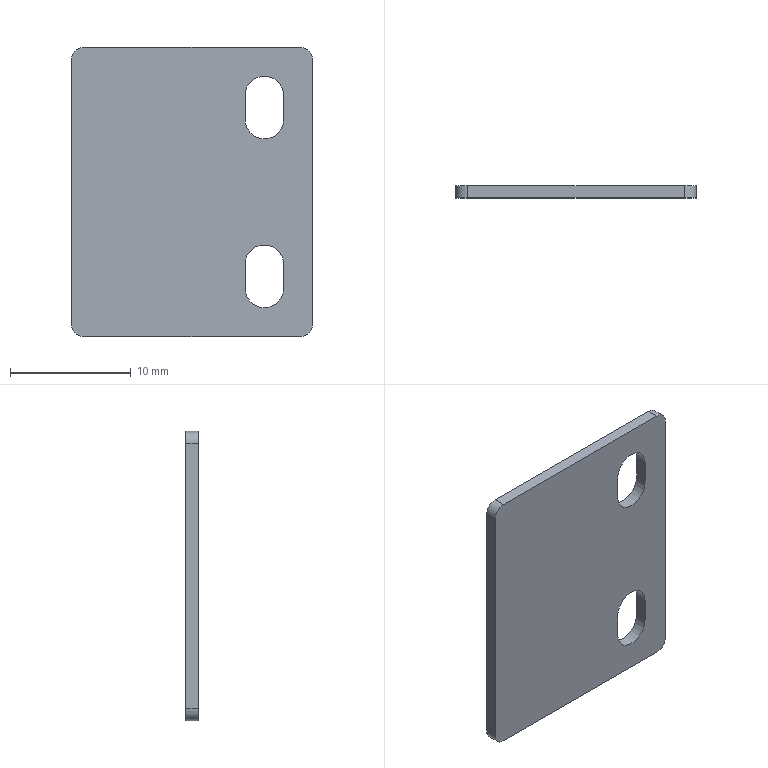Part | STEP file | QA-AD20 | 1 solid | 20 faces | box 20 x 1 x 24 mm | volume 450.257 mm3 | cylinder 10 | plane 10 | commonest cylinder face diameters 3.2 x6 2 x4